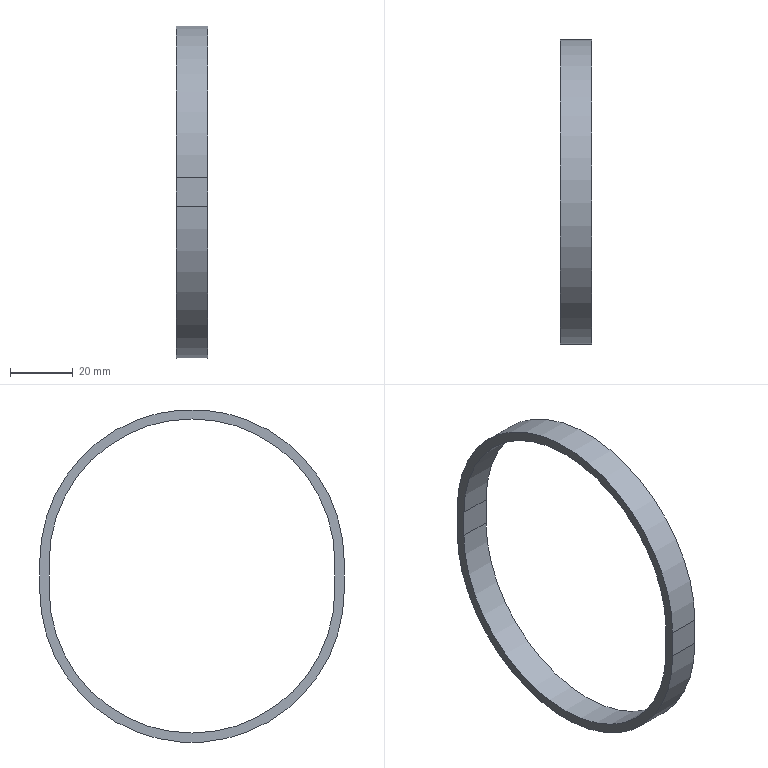Part | STEP file | 1-56.12 | 1 solid | 10 faces | box 10 x 97 x 106 mm | volume 9399 mm3 | plane 6 | cylinder 4 | commonest cylinder face diameters 91 x2 97 x2
STEP:
#1=CARTESIAN_POINT('',(0.,0.,0.));
#2=DIRECTION('',(0.,0.,1.));
#3=DIRECTION('',(1.,0.,0.));
#4=AXIS2_PLACEMENT_3D('',#1,#2,#3);
#5=CARTESIAN_POINT('',(0.,-48.5,0.));
#6=VERTEX_POINT('',#5);
#7=CARTESIAN_POINT('',(0.,-48.5,-9.));
#8=VERTEX_POINT('',#7);
#9=CARTESIAN_POINT('',(0.,-48.5,0.));
#10=DIRECTION('',(0.,0.,-1.));
#11=VECTOR('',#10,1.);
#12=LINE('',#9,#11);
#13=CARTESIAN_POINT('',(0.,4.5,-4.5));
#14=DIRECTION('',(1.,0.,0.));
#15=DIRECTION('',(0.,1.,0.));
#16=AXIS2_PLACEMENT_3D('',#13,#14,#15);
#17=PLANE('',#16);
#18=CARTESIAN_POINT('',(-53.,4.5));
#19=DIRECTION('',(0.,-1.));
#20=VECTOR('',#19,1.);
#21=LINE('',#18,#20);
#22=(GEOMETRIC_REPRESENTATION_CONTEXT(2)PARAMETRIC_REPRESENTATION_CONTEXT()REPRESENTATION_CONTEXT('',''));
#23=DEFINITIONAL_REPRESENTATION('',(#21),#22);
#24=PCURVE('',#17,#23);
#25=CARTESIAN_POINT('',(5.,-48.5,-4.5));
#26=DIRECTION('',(0.,-1.,0.));
#27=DIRECTION('',(0.,0.,-1.));
#28=AXIS2_PLACEMENT_3D('',#25,#26,#27);
#29=PLANE('',#28);
#30=CARTESIAN_POINT('',(-4.5,-5.));
#31=DIRECTION('',(1.,0.));
#32=VECTOR('',#31,1.);
#33=LINE('',#30,#32);
#34=(GEOMETRIC_REPRESENTATION_CONTEXT(2)PARAMETRIC_REPRESENTATION_CONTEXT()REPRESENTATION_CONTEXT('',''));
#35=DEFINITIONAL_REPRESENTATION('',(#33),#34);
#36=PCURVE('',#29,#35);
#37=SURFACE_CURVE('',#12,(#24,#36),.PCURVE_S1.);
#38=EDGE_CURVE('',#6,#8,#37,.T.);
#39=ORIENTED_EDGE('',*,*,#38,.T.);
#40=CARTESIAN_POINT('',(0.,48.5,-9.));
#41=VERTEX_POINT('',#40);
#42=CARTESIAN_POINT('',(0.,0.,-9.));
#43=DIRECTION('',(1.,0.,0.));
#44=DIRECTION('',(0.,-1.,0.));
#45=AXIS2_PLACEMENT_3D('',#42,#43,#44);
#46=CIRCLE('',#45,48.5);
#47=CARTESIAN_POINT('',(-4.5,-4.5));
#48=DIRECTION('',(-1.,0.));
#49=AXIS2_PLACEMENT_2D('',#47,#48);
#50=CIRCLE('',#49,48.5);
#51=(GEOMETRIC_REPRESENTATION_CONTEXT(2)PARAMETRIC_REPRESENTATION_CONTEXT()REPRESENTATION_CONTEXT('',''));
#52=DEFINITIONAL_REPRESENTATION('',(#50),#51);
#53=PCURVE('',#17,#52);
#54=CARTESIAN_POINT('',(0.,0.,-9.));
#55=DIRECTION('',(1.,0.,0.));
#56=DIRECTION('',(0.,-1.,0.));
#57=AXIS2_PLACEMENT_3D('',#54,#55,#56);
#58=CYLINDRICAL_SURFACE('',#57,48.5);
#59=CARTESIAN_POINT('',(0.,0.));
#60=DIRECTION('',(1.,0.));
#61=VECTOR('',#60,1.);
#62=LINE('',#59,#61);
#63=(GEOMETRIC_REPRESENTATION_CONTEXT(2)PARAMETRIC_REPRESENTATION_CONTEXT()REPRESENTATION_CONTEXT('',''));
#64=DEFINITIONAL_REPRESENTATION('',(#62),#63);
#65=PCURVE('',#58,#64);
#66=SURFACE_CURVE('',#46,(#53,#65),.PCURVE_S1.);
#67=EDGE_CURVE('',#8,#41,#66,.T.);
#68=ORIENTED_EDGE('',*,*,#67,.T.);
#69=CARTESIAN_POINT('',(0.,48.5,0.));
#70=VERTEX_POINT('',#69);
#71=CARTESIAN_POINT('',(0.,48.5,-9.));
#72=DIRECTION('',(0.,0.,1.));
#73=VECTOR('',#72,1.);
#74=LINE('',#71,#73);
#75=CARTESIAN_POINT('',(44.,-4.5));
#76=DIRECTION('',(0.,1.));
#77=VECTOR('',#76,1.);
#78=LINE('',#75,#77);
#79=(GEOMETRIC_REPRESENTATION_CONTEXT(2)PARAMETRIC_REPRESENTATION_CONTEXT()REPRESENTATION_CONTEXT('',''));
#80=DEFINITIONAL_REPRESENTATION('',(#78),#79);
#81=PCURVE('',#17,#80);
#82=CARTESIAN_POINT('',(5.,48.5,-4.5));
#83=DIRECTION('',(0.,1.,0.));
#84=DIRECTION('',(0.,0.,1.));
#85=AXIS2_PLACEMENT_3D('',#82,#83,#84);
#86=PLANE('',#85);
#87=CARTESIAN_POINT('',(-4.5,-5.));
#88=DIRECTION('',(1.,0.));
#89=VECTOR('',#88,1.);
#90=LINE('',#87,#89);
#91=(GEOMETRIC_REPRESENTATION_CONTEXT(2)PARAMETRIC_REPRESENTATION_CONTEXT()REPRESENTATION_CONTEXT('',''));
#92=DEFINITIONAL_REPRESENTATION('',(#90),#91);
#93=PCURVE('',#86,#92);
#94=SURFACE_CURVE('',#74,(#81,#93),.PCURVE_S1.);
#95=EDGE_CURVE('',#41,#70,#94,.T.);
#96=ORIENTED_EDGE('',*,*,#95,.T.);
#97=CARTESIAN_POINT('',(0.,0.,0.));
#98=DIRECTION('',(1.,0.,0.));
#99=DIRECTION('',(0.,1.,0.));
#100=AXIS2_PLACEMENT_3D('',#97,#98,#99);
#101=CIRCLE('',#100,48.5);
#102=CARTESIAN_POINT('',(-4.5,4.5));
#103=DIRECTION('',(1.,0.));
#104=AXIS2_PLACEMENT_2D('',#102,#103);
#105=CIRCLE('',#104,48.5);
#106=(GEOMETRIC_REPRESENTATION_CONTEXT(2)PARAMETRIC_REPRESENTATION_CONTEXT()REPRESENTATION_CONTEXT('',''));
#107=DEFINITIONAL_REPRESENTATION('',(#105),#106);
#108=PCURVE('',#17,#107);
#109=CARTESIAN_POINT('',(0.,0.,0.));
#110=DIRECTION('',(1.,0.,0.));
#111=DIRECTION('',(0.,1.,0.));
#112=AXIS2_PLACEMENT_3D('',#109,#110,#111);
#113=CYLINDRICAL_SURFACE('',#112,48.5);
#114=CARTESIAN_POINT('',(0.,0.));
#115=DIRECTION('',(1.,0.));
#116=VECTOR('',#115,1.);
#117=LINE('',#114,#116);
#118=(GEOMETRIC_REPRESENTATION_CONTEXT(2)PARAMETRIC_REPRESENTATION_CONTEXT()REPRESENTATION_CONTEXT('',''));
#119=DEFINITIONAL_REPRESENTATION('',(#117),#118);
#120=PCURVE('',#113,#119);
#121=SURFACE_CURVE('',#101,(#108,#120),.PCURVE_S1.);
#122=EDGE_CURVE('',#70,#6,#121,.T.);
#123=ORIENTED_EDGE('',*,*,#122,.T.);
#124=EDGE_LOOP('',(#39,#68,#96,#123));
#125=FACE_BOUND('',#124,.F.);
#126=CARTESIAN_POINT('',(0.,45.5,0.));
#127=VERTEX_POINT('',#126);
#128=CARTESIAN_POINT('',(0.,45.5,-9.));
#129=VERTEX_POINT('',#128);
#130=CARTESIAN_POINT('',(0.,45.5,0.));
#131=DIRECTION('',(0.,0.,-1.));
#132=VECTOR('',#131,1.);
#133=LINE('',#130,#132);
#134=CARTESIAN_POINT('',(41.,4.5));
#135=DIRECTION('',(0.,-1.));
#136=VECTOR('',#135,1.);
#137=LINE('',#134,#136);
#138=(GEOMETRIC_REPRESENTATION_CONTEXT(2)PARAMETRIC_REPRESENTATION_CONTEXT()REPRESENTATION_CONTEXT('',''));
#139=DEFINITIONAL_REPRESENTATION('',(#137),#138);
#140=PCURVE('',#17,#139);
#141=CARTESIAN_POINT('',(5.,45.5,-4.5));
#142=DIRECTION('',(0.,-1.,0.));
#143=DIRECTION('',(0.,0.,-1.));
#144=AXIS2_PLACEMENT_3D('',#141,#142,#143);
#145=PLANE('',#144);
#146=CARTESIAN_POINT('',(-4.5,-5.));
#147=DIRECTION('',(1.,0.));
#148=VECTOR('',#147,1.);
#149=LINE('',#146,#148);
#150=(GEOMETRIC_REPRESENTATION_CONTEXT(2)PARAMETRIC_REPRESENTATION_CONTEXT()REPRESENTATION_CONTEXT('',''));
#151=DEFINITIONAL_REPRESENTATION('',(#149),#150);
#152=PCURVE('',#145,#151);
#153=SURFACE_CURVE('',#133,(#140,#152),.PCURVE_S1.);
#154=EDGE_CURVE('',#127,#129,#153,.T.);
#155=ORIENTED_EDGE('',*,*,#154,.T.);
#156=CARTESIAN_POINT('',(0.,-45.5,-9.));
#157=VERTEX_POINT('',#156);
#158=CARTESIAN_POINT('',(0.,0.,-9.));
#159=DIRECTION('',(-1.,0.,0.));
#160=DIRECTION('',(0.,1.,0.));
#161=AXIS2_PLACEMENT_3D('',#158,#159,#160);
#162=CIRCLE('',#161,45.5);
#163=CARTESIAN_POINT('',(41.,-4.5));
#164=CARTESIAN_POINT('',(41.,-83.308));
#165=CARTESIAN_POINT('',(-27.25,-43.904));
#166=CARTESIAN_POINT('',(-95.5,-4.5));
#167=CARTESIAN_POINT('',(-27.25,34.904));
#168=CARTESIAN_POINT('',(41.,74.308));
#169=CARTESIAN_POINT('',(41.,-4.5));
#170=(BOUNDED_CURVE()B_SPLINE_CURVE(2,(#163,#164,#165,#166,#167,#168,#169),.UNSPECIFIED.,.T.,.F.)B_SPLINE_CURVE_WITH_KNOTS((1,2,2,2,2,1),(-2.094,0.,2.094,4.189,6.283,8.378),.UNSPECIFIED.)CURVE()GEOMETRIC_REPRESENTATION_ITEM()RATIONAL_B_SPLINE_CURVE((1.,0.5,1.,0.5,1.,0.5,1.))REPRESENTATION_ITEM(''));
#171=(GEOMETRIC_REPRESENTATION_CONTEXT(2)PARAMETRIC_REPRESENTATION_CONTEXT()REPRESENTATION_CONTEXT('',''));
#172=DEFINITIONAL_REPRESENTATION('',(#170),#171);
#173=PCURVE('',#17,#172);
#174=CARTESIAN_POINT('',(0.,0.,-9.));
#175=DIRECTION('',(1.,0.,0.));
#176=DIRECTION('',(0.,1.,0.));
#177=AXIS2_PLACEMENT_3D('',#174,#175,#176);
#178=CYLINDRICAL_SURFACE('',#177,45.5);
#179=CARTESIAN_POINT('',(6.283,0.));
#180=DIRECTION('',(-1.,0.));
#181=VECTOR('',#180,1.);
#182=LINE('',#179,#181);
#183=(GEOMETRIC_REPRESENTATION_CONTEXT(2)PARAMETRIC_REPRESENTATION_CONTEXT()REPRESENTATION_CONTEXT('',''));
#184=DEFINITIONAL_REPRESENTATION('',(#182),#183);
#185=PCURVE('',#178,#184);
#186=SURFACE_CURVE('',#162,(#173,#185),.PCURVE_S1.);
#187=EDGE_CURVE('',#129,#157,#186,.T.);
#188=ORIENTED_EDGE('',*,*,#187,.T.);
#189=CARTESIAN_POINT('',(0.,-45.5,0.));
#190=VERTEX_POINT('',#189);
#191=CARTESIAN_POINT('',(0.,-45.5,-9.));
#192=DIRECTION('',(0.,0.,1.));
#193=VECTOR('',#192,1.);
#194=LINE('',#191,#193);
#195=CARTESIAN_POINT('',(-50.,-4.5));
#196=DIRECTION('',(0.,1.));
#197=VECTOR('',#196,1.);
#198=LINE('',#195,#197);
#199=(GEOMETRIC_REPRESENTATION_CONTEXT(2)PARAMETRIC_REPRESENTATION_CONTEXT()REPRESENTATION_CONTEXT('',''));
#200=DEFINITIONAL_REPRESENTATION('',(#198),#199);
#201=PCURVE('',#17,#200);
#202=CARTESIAN_POINT('',(5.,-45.5,-4.5));
#203=DIRECTION('',(0.,1.,0.));
#204=DIRECTION('',(0.,0.,1.));
#205=AXIS2_PLACEMENT_3D('',#202,#203,#204);
#206=PLANE('',#205);
#207=CARTESIAN_POINT('',(-4.5,-5.));
#208=DIRECTION('',(1.,0.));
#209=VECTOR('',#208,1.);
#210=LINE('',#207,#209);
#211=(GEOMETRIC_REPRESENTATION_CONTEXT(2)PARAMETRIC_REPRESENTATION_CONTEXT()REPRESENTATION_CONTEXT('',''));
#212=DEFINITIONAL_REPRESENTATION('',(#210),#211);
#213=PCURVE('',#206,#212);
#214=SURFACE_CURVE('',#194,(#201,#213),.PCURVE_S1.);
#215=EDGE_CURVE('',#157,#190,#214,.T.);
#216=ORIENTED_EDGE('',*,*,#215,.T.);
#217=CARTESIAN_POINT('',(0.,0.,0.));
#218=DIRECTION('',(-1.,0.,0.));
#219=DIRECTION('',(0.,-1.,0.));
#220=AXIS2_PLACEMENT_3D('',#217,#218,#219);
#221=CIRCLE('',#220,45.5);
#222=CARTESIAN_POINT('',(-50.,4.5));
#223=CARTESIAN_POINT('',(-50.,83.308));
#224=CARTESIAN_POINT('',(18.25,43.904));
#225=CARTESIAN_POINT('',(86.5,4.5));
#226=CARTESIAN_POINT('',(18.25,-34.904));
#227=CARTESIAN_POINT('',(-50.,-74.308));
#228=CARTESIAN_POINT('',(-50.,4.5));
#229=(BOUNDED_CURVE()B_SPLINE_CURVE(2,(#222,#223,#224,#225,#226,#227,#228),.UNSPECIFIED.,.T.,.F.)B_SPLINE_CURVE_WITH_KNOTS((1,2,2,2,2,1),(-2.094,0.,2.094,4.189,6.283,8.378),.UNSPECIFIED.)CURVE()GEOMETRIC_REPRESENTATION_ITEM()RATIONAL_B_SPLINE_CURVE((1.,0.5,1.,0.5,1.,0.5,1.))REPRESENTATION_ITEM(''));
#230=(GEOMETRIC_REPRESENTATION_CONTEXT(2)PARAMETRIC_REPRESENTATION_CONTEXT()REPRESENTATION_CONTEXT('',''));
#231=DEFINITIONAL_REPRESENTATION('',(#229),#230);
#232=PCURVE('',#17,#231);
#233=CARTESIAN_POINT('',(0.,0.,0.));
#234=DIRECTION('',(1.,0.,0.));
#235=DIRECTION('',(0.,-1.,0.));
#236=AXIS2_PLACEMENT_3D('',#233,#234,#235);
#237=CYLINDRICAL_SURFACE('',#236,45.5);
#238=CARTESIAN_POINT('',(6.283,0.));
#239=DIRECTION('',(-1.,0.));
#240=VECTOR('',#239,1.);
#241=LINE('',#238,#240);
#242=(GEOMETRIC_REPRESENTATION_CONTEXT(2)PARAMETRIC_REPRESENTATION_CONTEXT()REPRESENTATION_CONTEXT('',''));
#243=DEFINITIONAL_REPRESENTATION('',(#241),#242);
#244=PCURVE('',#237,#243);
#245=SURFACE_CURVE('',#221,(#232,#244),.PCURVE_S1.);
#246=EDGE_CURVE('',#190,#127,#245,.T.);
#247=ORIENTED_EDGE('',*,*,#246,.T.);
#248=EDGE_LOOP('',(#155,#188,#216,#247));
#249=FACE_BOUND('',#248,.F.);
#250=ADVANCED_FACE('',(#125,#249),#17,.F.);
#251=CARTESIAN_POINT('',(10.,-48.5,0.));
#252=VERTEX_POINT('',#251);
#253=CARTESIAN_POINT('',(10.,-48.5,-9.));
#254=VERTEX_POINT('',#253);
#255=CARTESIAN_POINT('',(10.,-48.5,0.));
#256=DIRECTION('',(0.,0.,-1.));
#257=VECTOR('',#256,1.);
#258=LINE('',#255,#257);
#259=CARTESIAN_POINT('',(10.,4.5,-4.5));
#260=DIRECTION('',(1.,0.,0.));
#261=DIRECTION('',(0.,1.,0.));
#262=AXIS2_PLACEMENT_3D('',#259,#260,#261);
#263=PLANE('',#262);
#264=CARTESIAN_POINT('',(-53.,4.5));
#265=DIRECTION('',(0.,-1.));
#266=VECTOR('',#265,1.);
#267=LINE('',#264,#266);
#268=(GEOMETRIC_REPRESENTATION_CONTEXT(2)PARAMETRIC_REPRESENTATION_CONTEXT()REPRESENTATION_CONTEXT('',''));
#269=DEFINITIONAL_REPRESENTATION('',(#267),#268);
#270=PCURVE('',#263,#269);
#271=CARTESIAN_POINT('',(-4.5,5.));
#272=DIRECTION('',(1.,0.));
#273=VECTOR('',#272,1.);
#274=LINE('',#271,#273);
#275=(GEOMETRIC_REPRESENTATION_CONTEXT(2)PARAMETRIC_REPRESENTATION_CONTEXT()REPRESENTATION_CONTEXT('',''));
#276=DEFINITIONAL_REPRESENTATION('',(#274),#275);
#277=PCURVE('',#29,#276);
#278=SURFACE_CURVE('',#258,(#270,#277),.PCURVE_S1.);
#279=EDGE_CURVE('',#252,#254,#278,.T.);
#280=ORIENTED_EDGE('',*,*,#279,.T.);
#281=CARTESIAN_POINT('',(10.,48.5,-9.));
#282=VERTEX_POINT('',#281);
#283=CARTESIAN_POINT('',(10.,0.,-9.));
#284=DIRECTION('',(1.,0.,0.));
#285=DIRECTION('',(0.,-1.,0.));
#286=AXIS2_PLACEMENT_3D('',#283,#284,#285);
#287=CIRCLE('',#286,48.5);
#288=CARTESIAN_POINT('',(-4.5,-4.5));
#289=DIRECTION('',(-1.,0.));
#290=AXIS2_PLACEMENT_2D('',#288,#289);
#291=CIRCLE('',#290,48.5);
#292=(GEOMETRIC_REPRESENTATION_CONTEXT(2)PARAMETRIC_REPRESENTATION_CONTEXT()REPRESENTATION_CONTEXT('',''));
#293=DEFINITIONAL_REPRESENTATION('',(#291),#292);
#294=PCURVE('',#263,#293);
#295=CARTESIAN_POINT('',(0.,10.));
#296=DIRECTION('',(1.,0.));
#297=VECTOR('',#296,1.);
#298=LINE('',#295,#297);
#299=(GEOMETRIC_REPRESENTATION_CONTEXT(2)PARAMETRIC_REPRESENTATION_CONTEXT()REPRESENTATION_CONTEXT('',''));
#300=DEFINITIONAL_REPRESENTATION('',(#298),#299);
#301=PCURVE('',#58,#300);
#302=SURFACE_CURVE('',#287,(#294,#301),.PCURVE_S1.);
#303=EDGE_CURVE('',#254,#282,#302,.T.);
#304=ORIENTED_EDGE('',*,*,#303,.T.);
#305=CARTESIAN_POINT('',(10.,48.5,0.));
#306=VERTEX_POINT('',#305);
#307=CARTESIAN_POINT('',(10.,48.5,-9.));
#308=DIRECTION('',(0.,0.,1.));
#309=VECTOR('',#308,1.);
#310=LINE('',#307,#309);
#311=CARTESIAN_POINT('',(44.,-4.5));
#312=DIRECTION('',(0.,1.));
#313=VECTOR('',#312,1.);
#314=LINE('',#311,#313);
#315=(GEOMETRIC_REPRESENTATION_CONTEXT(2)PARAMETRIC_REPRESENTATION_CONTEXT()REPRESENTATION_CONTEXT('',''));
#316=DEFINITIONAL_REPRESENTATION('',(#314),#315);
#317=PCURVE('',#263,#316);
#318=CARTESIAN_POINT('',(-4.5,5.));
#319=DIRECTION('',(1.,0.));
#320=VECTOR('',#319,1.);
#321=LINE('',#318,#320);
#322=(GEOMETRIC_REPRESENTATION_CONTEXT(2)PARAMETRIC_REPRESENTATION_CONTEXT()REPRESENTATION_CONTEXT('',''));
#323=DEFINITIONAL_REPRESENTATION('',(#321),#322);
#324=PCURVE('',#86,#323);
#325=SURFACE_CURVE('',#310,(#317,#324),.PCURVE_S1.);
#326=EDGE_CURVE('',#282,#306,#325,.T.);
#327=ORIENTED_EDGE('',*,*,#326,.T.);
#328=CARTESIAN_POINT('',(10.,0.,0.));
#329=DIRECTION('',(1.,0.,0.));
#330=DIRECTION('',(0.,1.,0.));
#331=AXIS2_PLACEMENT_3D('',#328,#329,#330);
#332=CIRCLE('',#331,48.5);
#333=CARTESIAN_POINT('',(-4.5,4.5));
#334=DIRECTION('',(1.,0.));
#335=AXIS2_PLACEMENT_2D('',#333,#334);
#336=CIRCLE('',#335,48.5);
#337=(GEOMETRIC_REPRESENTATION_CONTEXT(2)PARAMETRIC_REPRESENTATION_CONTEXT()REPRESENTATION_CONTEXT('',''));
#338=DEFINITIONAL_REPRESENTATION('',(#336),#337);
#339=PCURVE('',#263,#338);
#340=CARTESIAN_POINT('',(0.,10.));
#341=DIRECTION('',(1.,0.));
#342=VECTOR('',#341,1.);
#343=LINE('',#340,#342);
#344=(GEOMETRIC_REPRESENTATION_CONTEXT(2)PARAMETRIC_REPRESENTATION_CONTEXT()REPRESENTATION_CONTEXT('',''));
#345=DEFINITIONAL_REPRESENTATION('',(#343),#344);
#346=PCURVE('',#113,#345);
#347=SURFACE_CURVE('',#332,(#339,#346),.PCURVE_S1.);
#348=EDGE_CURVE('',#306,#252,#347,.T.);
#349=ORIENTED_EDGE('',*,*,#348,.T.);
#350=EDGE_LOOP('',(#280,#304,#327,#349));
#351=FACE_BOUND('',#350,.T.);
#352=CARTESIAN_POINT('',(10.,45.5,0.));
#353=VERTEX_POINT('',#352);
#354=CARTESIAN_POINT('',(10.,45.5,-9.));
#355=VERTEX_POINT('',#354);
#356=CARTESIAN_POINT('',(10.,45.5,0.));
#357=DIRECTION('',(0.,0.,-1.));
#358=VECTOR('',#357,1.);
#359=LINE('',#356,#358);
#360=CARTESIAN_POINT('',(41.,4.5));
#361=DIRECTION('',(0.,-1.));
#362=VECTOR('',#361,1.);
#363=LINE('',#360,#362);
#364=(GEOMETRIC_REPRESENTATION_CONTEXT(2)PARAMETRIC_REPRESENTATION_CONTEXT()REPRESENTATION_CONTEXT('',''));
#365=DEFINITIONAL_REPRESENTATION('',(#363),#364);
#366=PCURVE('',#263,#365);
#367=CARTESIAN_POINT('',(-4.5,5.));
#368=DIRECTION('',(1.,0.));
#369=VECTOR('',#368,1.);
#370=LINE('',#367,#369);
#371=(GEOMETRIC_REPRESENTATION_CONTEXT(2)PARAMETRIC_REPRESENTATION_CONTEXT()REPRESENTATION_CONTEXT('',''));
#372=DEFINITIONAL_REPRESENTATION('',(#370),#371);
#373=PCURVE('',#145,#372);
#374=SURFACE_CURVE('',#359,(#366,#373),.PCURVE_S1.);
#375=EDGE_CURVE('',#353,#355,#374,.T.);
#376=ORIENTED_EDGE('',*,*,#375,.T.);
#377=CARTESIAN_POINT('',(10.,-45.5,-9.));
#378=VERTEX_POINT('',#377);
#379=CARTESIAN_POINT('',(10.,0.,-9.));
#380=DIRECTION('',(-1.,0.,0.));
#381=DIRECTION('',(0.,1.,0.));
#382=AXIS2_PLACEMENT_3D('',#379,#380,#381);
#383=CIRCLE('',#382,45.5);
#384=CARTESIAN_POINT('',(41.,-4.5));
#385=CARTESIAN_POINT('',(41.,-83.308));
#386=CARTESIAN_POINT('',(-27.25,-43.904));
#387=CARTESIAN_POINT('',(-95.5,-4.5));
#388=CARTESIAN_POINT('',(-27.25,34.904));
#389=CARTESIAN_POINT('',(41.,74.308));
#390=CARTESIAN_POINT('',(41.,-4.5));
#391=(BOUNDED_CURVE()B_SPLINE_CURVE(2,(#384,#385,#386,#387,#388,#389,#390),.UNSPECIFIED.,.T.,.F.)B_SPLINE_CURVE_WITH_KNOTS((1,2,2,2,2,1),(-2.094,0.,2.094,4.189,6.283,8.378),.UNSPECIFIED.)CURVE()GEOMETRIC_REPRESENTATION_ITEM()RATIONAL_B_SPLINE_CURVE((1.,0.5,1.,0.5,1.,0.5,1.))REPRESENTATION_ITEM(''));
#392=(GEOMETRIC_REPRESENTATION_CONTEXT(2)PARAMETRIC_REPRESENTATION_CONTEXT()REPRESENTATION_CONTEXT('',''));
#393=DEFINITIONAL_REPRESENTATION('',(#391),#392);
#394=PCURVE('',#263,#393);
#395=CARTESIAN_POINT('',(6.283,10.));
#396=DIRECTION('',(-1.,0.));
#397=VECTOR('',#396,1.);
#398=LINE('',#395,#397);
#399=(GEOMETRIC_REPRESENTATION_CONTEXT(2)PARAMETRIC_REPRESENTATION_CONTEXT()REPRESENTATION_CONTEXT('',''));
#400=DEFINITIONAL_REPRESENTATION('',(#398),#399);
#401=PCURVE('',#178,#400);
#402=SURFACE_CURVE('',#383,(#394,#401),.PCURVE_S1.);
#403=EDGE_CURVE('',#355,#378,#402,.T.);
#404=ORIENTED_EDGE('',*,*,#403,.T.);
#405=CARTESIAN_POINT('',(10.,-45.5,0.));
#406=VERTEX_POINT('',#405);
#407=CARTESIAN_POINT('',(10.,-45.5,-9.));
#408=DIRECTION('',(0.,0.,1.));
#409=VECTOR('',#408,1.);
#410=LINE('',#407,#409);
#411=CARTESIAN_POINT('',(-50.,-4.5));
#412=DIRECTION('',(0.,1.));
#413=VECTOR('',#412,1.);
#414=LINE('',#411,#413);
#415=(GEOMETRIC_REPRESENTATION_CONTEXT(2)PARAMETRIC_REPRESENTATION_CONTEXT()REPRESENTATION_CONTEXT('',''));
#416=DEFINITIONAL_REPRESENTATION('',(#414),#415);
#417=PCURVE('',#263,#416);
#418=CARTESIAN_POINT('',(-4.5,5.));
#419=DIRECTION('',(1.,0.));
#420=VECTOR('',#419,1.);
#421=LINE('',#418,#420);
#422=(GEOMETRIC_REPRESENTATION_CONTEXT(2)PARAMETRIC_REPRESENTATION_CONTEXT()REPRESENTATION_CONTEXT('',''));
#423=DEFINITIONAL_REPRESENTATION('',(#421),#422);
#424=PCURVE('',#206,#423);
#425=SURFACE_CURVE('',#410,(#417,#424),.PCURVE_S1.);
#426=EDGE_CURVE('',#378,#406,#425,.T.);
#427=ORIENTED_EDGE('',*,*,#426,.T.);
#428=CARTESIAN_POINT('',(10.,0.,0.));
#429=DIRECTION('',(-1.,0.,0.));
#430=DIRECTION('',(0.,-1.,0.));
#431=AXIS2_PLACEMENT_3D('',#428,#429,#430);
#432=CIRCLE('',#431,45.5);
#433=CARTESIAN_POINT('',(-50.,4.5));
#434=CARTESIAN_POINT('',(-50.,83.308));
#435=CARTESIAN_POINT('',(18.25,43.904));
#436=CARTESIAN_POINT('',(86.5,4.5));
#437=CARTESIAN_POINT('',(18.25,-34.904));
#438=CARTESIAN_POINT('',(-50.,-74.308));
#439=CARTESIAN_POINT('',(-50.,4.5));
#440=(BOUNDED_CURVE()B_SPLINE_CURVE(2,(#433,#434,#435,#436,#437,#438,#439),.UNSPECIFIED.,.T.,.F.)B_SPLINE_CURVE_WITH_KNOTS((1,2,2,2,2,1),(-2.094,0.,2.094,4.189,6.283,8.378),.UNSPECIFIED.)CURVE()GEOMETRIC_REPRESENTATION_ITEM()RATIONAL_B_SPLINE_CURVE((1.,0.5,1.,0.5,1.,0.5,1.))REPRESENTATION_ITEM(''));
#441=(GEOMETRIC_REPRESENTATION_CONTEXT(2)PARAMETRIC_REPRESENTATION_CONTEXT()REPRESENTATION_CONTEXT('',''));
#442=DEFINITIONAL_REPRESENTATION('',(#440),#441);
#443=PCURVE('',#263,#442);
#444=CARTESIAN_POINT('',(6.283,10.));
#445=DIRECTION('',(-1.,0.));
#446=VECTOR('',#445,1.);
#447=LINE('',#444,#446);
#448=(GEOMETRIC_REPRESENTATION_CONTEXT(2)PARAMETRIC_REPRESENTATION_CONTEXT()REPRESENTATION_CONTEXT('',''));
#449=DEFINITIONAL_REPRESENTATION('',(#447),#448);
#450=PCURVE('',#237,#449);
#451=SURFACE_CURVE('',#432,(#443,#450),.PCURVE_S1.);
#452=EDGE_CURVE('',#406,#353,#451,.T.);
#453=ORIENTED_EDGE('',*,*,#452,.T.);
#454=EDGE_LOOP('',(#376,#404,#427,#453));
#455=FACE_BOUND('',#454,.T.);
#456=ADVANCED_FACE('',(#351,#455),#263,.T.);
#457=ORIENTED_EDGE('',*,*,#38,.T.);
#458=CARTESIAN_POINT('',(0.,-48.5,-9.));
#459=DIRECTION('',(1.,0.,0.));
#460=VECTOR('',#459,1.);
#461=LINE('',#458,#460);
#462=CARTESIAN_POINT('',(4.5,-5.));
#463=DIRECTION('',(0.,1.));
#464=VECTOR('',#463,1.);
#465=LINE('',#462,#464);
#466=(GEOMETRIC_REPRESENTATION_CONTEXT(2)PARAMETRIC_REPRESENTATION_CONTEXT()REPRESENTATION_CONTEXT('',''));
#467=DEFINITIONAL_REPRESENTATION('',(#465),#466);
#468=PCURVE('',#29,#467);
#469=CARTESIAN_POINT('',(0.,0.));
#470=DIRECTION('',(0.,1.));
#471=VECTOR('',#470,1.);
#472=LINE('',#469,#471);
#473=(GEOMETRIC_REPRESENTATION_CONTEXT(2)PARAMETRIC_REPRESENTATION_CONTEXT()REPRESENTATION_CONTEXT('',''));
#474=DEFINITIONAL_REPRESENTATION('',(#472),#473);
#475=PCURVE('',#58,#474);
#476=SURFACE_CURVE('',#461,(#468,#475),.PCURVE_S1.);
#477=EDGE_CURVE('',#8,#254,#476,.T.);
#478=ORIENTED_EDGE('',*,*,#477,.T.);
#479=ORIENTED_EDGE('',*,*,#279,.F.);
#480=CARTESIAN_POINT('',(0.,-48.5,0.));
#481=DIRECTION('',(1.,0.,0.));
#482=VECTOR('',#481,1.);
#483=LINE('',#480,#482);
#484=CARTESIAN_POINT('',(-4.5,-5.));
#485=DIRECTION('',(0.,1.));
#486=VECTOR('',#485,1.);
#487=LINE('',#484,#486);
#488=(GEOMETRIC_REPRESENTATION_CONTEXT(2)PARAMETRIC_REPRESENTATION_CONTEXT()REPRESENTATION_CONTEXT('',''));
#489=DEFINITIONAL_REPRESENTATION('',(#487),#488);
#490=PCURVE('',#29,#489);
#491=CARTESIAN_POINT('',(3.142,0.));
#492=DIRECTION('',(0.,1.));
#493=VECTOR('',#492,1.);
#494=LINE('',#491,#493);
#495=(GEOMETRIC_REPRESENTATION_CONTEXT(2)PARAMETRIC_REPRESENTATION_CONTEXT()REPRESENTATION_CONTEXT('',''));
#496=DEFINITIONAL_REPRESENTATION('',(#494),#495);
#497=PCURVE('',#113,#496);
#498=SURFACE_CURVE('',#483,(#490,#497),.PCURVE_S1.);
#499=EDGE_CURVE('',#6,#252,#498,.T.);
#500=ORIENTED_EDGE('',*,*,#499,.F.);
#501=EDGE_LOOP('',(#457,#478,#479,#500));
#502=FACE_BOUND('',#501,.T.);
#503=ADVANCED_FACE('',(#502),#29,.T.);
#504=ORIENTED_EDGE('',*,*,#67,.T.);
#505=CARTESIAN_POINT('',(0.,48.5,-9.));
#506=DIRECTION('',(1.,0.,0.));
#507=VECTOR('',#506,1.);
#508=LINE('',#505,#507);
#509=CARTESIAN_POINT('',(3.142,0.));
#510=DIRECTION('',(0.,1.));
#511=VECTOR('',#510,1.);
#512=LINE('',#509,#511);
#513=(GEOMETRIC_REPRESENTATION_CONTEXT(2)PARAMETRIC_REPRESENTATION_CONTEXT()REPRESENTATION_CONTEXT('',''));
#514=DEFINITIONAL_REPRESENTATION('',(#512),#513);
#515=PCURVE('',#58,#514);
#516=CARTESIAN_POINT('',(-4.5,-5.));
#517=DIRECTION('',(0.,1.));
#518=VECTOR('',#517,1.);
#519=LINE('',#516,#518);
#520=(GEOMETRIC_REPRESENTATION_CONTEXT(2)PARAMETRIC_REPRESENTATION_CONTEXT()REPRESENTATION_CONTEXT('',''));
#521=DEFINITIONAL_REPRESENTATION('',(#519),#520);
#522=PCURVE('',#86,#521);
#523=SURFACE_CURVE('',#508,(#515,#522),.PCURVE_S1.);
#524=EDGE_CURVE('',#41,#282,#523,.T.);
#525=ORIENTED_EDGE('',*,*,#524,.T.);
#526=ORIENTED_EDGE('',*,*,#303,.F.);
#527=ORIENTED_EDGE('',*,*,#477,.F.);
#528=EDGE_LOOP('',(#504,#525,#526,#527));
#529=FACE_BOUND('',#528,.T.);
#530=ADVANCED_FACE('',(#529),#58,.T.);
#531=ORIENTED_EDGE('',*,*,#95,.T.);
#532=CARTESIAN_POINT('',(0.,48.5,0.));
#533=DIRECTION('',(1.,0.,0.));
#534=VECTOR('',#533,1.);
#535=LINE('',#532,#534);
#536=CARTESIAN_POINT('',(4.5,-5.));
#537=DIRECTION('',(0.,1.));
#538=VECTOR('',#537,1.);
#539=LINE('',#536,#538);
#540=(GEOMETRIC_REPRESENTATION_CONTEXT(2)PARAMETRIC_REPRESENTATION_CONTEXT()REPRESENTATION_CONTEXT('',''));
#541=DEFINITIONAL_REPRESENTATION('',(#539),#540);
#542=PCURVE('',#86,#541);
#543=CARTESIAN_POINT('',(0.,0.));
#544=DIRECTION('',(0.,1.));
#545=VECTOR('',#544,1.);
#546=LINE('',#543,#545);
#547=(GEOMETRIC_REPRESENTATION_CONTEXT(2)PARAMETRIC_REPRESENTATION_CONTEXT()REPRESENTATION_CONTEXT('',''));
#548=DEFINITIONAL_REPRESENTATION('',(#546),#547);
#549=PCURVE('',#113,#548);
#550=SURFACE_CURVE('',#535,(#542,#549),.PCURVE_S1.);
#551=EDGE_CURVE('',#70,#306,#550,.T.);
#552=ORIENTED_EDGE('',*,*,#551,.T.);
#553=ORIENTED_EDGE('',*,*,#326,.F.);
#554=ORIENTED_EDGE('',*,*,#524,.F.);
#555=EDGE_LOOP('',(#531,#552,#553,#554));
#556=FACE_BOUND('',#555,.T.);
#557=ADVANCED_FACE('',(#556),#86,.T.);
#558=ORIENTED_EDGE('',*,*,#122,.T.);
#559=ORIENTED_EDGE('',*,*,#499,.T.);
#560=ORIENTED_EDGE('',*,*,#348,.F.);
#561=ORIENTED_EDGE('',*,*,#551,.F.);
#562=EDGE_LOOP('',(#558,#559,#560,#561));
#563=FACE_BOUND('',#562,.T.);
#564=ADVANCED_FACE('',(#563),#113,.T.);
#565=ORIENTED_EDGE('',*,*,#154,.T.);
#566=CARTESIAN_POINT('',(0.,45.5,-9.));
#567=DIRECTION('',(1.,0.,0.));
#568=VECTOR('',#567,1.);
#569=LINE('',#566,#568);
#570=CARTESIAN_POINT('',(4.5,-5.));
#571=DIRECTION('',(0.,1.));
#572=VECTOR('',#571,1.);
#573=LINE('',#570,#572);
#574=(GEOMETRIC_REPRESENTATION_CONTEXT(2)PARAMETRIC_REPRESENTATION_CONTEXT()REPRESENTATION_CONTEXT('',''));
#575=DEFINITIONAL_REPRESENTATION('',(#573),#574);
#576=PCURVE('',#145,#575);
#577=CARTESIAN_POINT('',(6.283,0.));
#578=DIRECTION('',(0.,1.));
#579=VECTOR('',#578,1.);
#580=LINE('',#577,#579);
#581=(GEOMETRIC_REPRESENTATION_CONTEXT(2)PARAMETRIC_REPRESENTATION_CONTEXT()REPRESENTATION_CONTEXT('',''));
#582=DEFINITIONAL_REPRESENTATION('',(#580),#581);
#583=PCURVE('',#178,#582);
#584=SURFACE_CURVE('',#569,(#576,#583),.PCURVE_S1.);
#585=EDGE_CURVE('',#129,#355,#584,.T.);
#586=ORIENTED_EDGE('',*,*,#585,.T.);
#587=ORIENTED_EDGE('',*,*,#375,.F.);
#588=CARTESIAN_POINT('',(0.,45.5,0.));
#589=DIRECTION('',(1.,0.,0.));
#590=VECTOR('',#589,1.);
#591=LINE('',#588,#590);
#592=CARTESIAN_POINT('',(-4.5,-5.));
#593=DIRECTION('',(0.,1.));
#594=VECTOR('',#593,1.);
#595=LINE('',#592,#594);
#596=(GEOMETRIC_REPRESENTATION_CONTEXT(2)PARAMETRIC_REPRESENTATION_CONTEXT()REPRESENTATION_CONTEXT('',''));
#597=DEFINITIONAL_REPRESENTATION('',(#595),#596);
#598=PCURVE('',#145,#597);
#599=CARTESIAN_POINT('',(3.142,0.));
#600=DIRECTION('',(0.,1.));
#601=VECTOR('',#600,1.);
#602=LINE('',#599,#601);
#603=(GEOMETRIC_REPRESENTATION_CONTEXT(2)PARAMETRIC_REPRESENTATION_CONTEXT()REPRESENTATION_CONTEXT('',''));
#604=DEFINITIONAL_REPRESENTATION('',(#602),#603);
#605=PCURVE('',#237,#604);
#606=SURFACE_CURVE('',#591,(#598,#605),.PCURVE_S1.);
#607=EDGE_CURVE('',#127,#353,#606,.T.);
#608=ORIENTED_EDGE('',*,*,#607,.F.);
#609=EDGE_LOOP('',(#565,#586,#587,#608));
#610=FACE_BOUND('',#609,.T.);
#611=ADVANCED_FACE('',(#610),#145,.T.);
#612=ORIENTED_EDGE('',*,*,#585,.T.);
#613=ORIENTED_EDGE('',*,*,#403,.T.);
#614=CARTESIAN_POINT('',(0.,-45.5,-9.));
#615=DIRECTION('',(1.,0.,0.));
#616=VECTOR('',#615,1.);
#617=LINE('',#614,#616);
#618=CARTESIAN_POINT('',(3.142,0.));
#619=DIRECTION('',(0.,1.));
#620=VECTOR('',#619,1.);
#621=LINE('',#618,#620);
#622=(GEOMETRIC_REPRESENTATION_CONTEXT(2)PARAMETRIC_REPRESENTATION_CONTEXT()REPRESENTATION_CONTEXT('',''));
#623=DEFINITIONAL_REPRESENTATION('',(#621),#622);
#624=PCURVE('',#178,#623);
#625=CARTESIAN_POINT('',(-4.5,-5.));
#626=DIRECTION('',(0.,1.));
#627=VECTOR('',#626,1.);
#628=LINE('',#625,#627);
#629=(GEOMETRIC_REPRESENTATION_CONTEXT(2)PARAMETRIC_REPRESENTATION_CONTEXT()REPRESENTATION_CONTEXT('',''));
#630=DEFINITIONAL_REPRESENTATION('',(#628),#629);
#631=PCURVE('',#206,#630);
#632=SURFACE_CURVE('',#617,(#624,#631),.PCURVE_S1.);
#633=EDGE_CURVE('',#157,#378,#632,.T.);
#634=ORIENTED_EDGE('',*,*,#633,.F.);
#635=ORIENTED_EDGE('',*,*,#187,.F.);
#636=EDGE_LOOP('',(#612,#613,#634,#635));
#637=FACE_BOUND('',#636,.F.);
#638=ADVANCED_FACE('',(#637),#178,.F.);
#639=ORIENTED_EDGE('',*,*,#215,.T.);
#640=CARTESIAN_POINT('',(0.,-45.5,0.));
#641=DIRECTION('',(1.,0.,0.));
#642=VECTOR('',#641,1.);
#643=LINE('',#640,#642);
#644=CARTESIAN_POINT('',(4.5,-5.));
#645=DIRECTION('',(0.,1.));
#646=VECTOR('',#645,1.);
#647=LINE('',#644,#646);
#648=(GEOMETRIC_REPRESENTATION_CONTEXT(2)PARAMETRIC_REPRESENTATION_CONTEXT()REPRESENTATION_CONTEXT('',''));
#649=DEFINITIONAL_REPRESENTATION('',(#647),#648);
#650=PCURVE('',#206,#649);
#651=CARTESIAN_POINT('',(6.283,0.));
#652=DIRECTION('',(0.,1.));
#653=VECTOR('',#652,1.);
#654=LINE('',#651,#653);
#655=(GEOMETRIC_REPRESENTATION_CONTEXT(2)PARAMETRIC_REPRESENTATION_CONTEXT()REPRESENTATION_CONTEXT('',''));
#656=DEFINITIONAL_REPRESENTATION('',(#654),#655);
#657=PCURVE('',#237,#656);
#658=SURFACE_CURVE('',#643,(#650,#657),.PCURVE_S1.);
#659=EDGE_CURVE('',#190,#406,#658,.T.);
#660=ORIENTED_EDGE('',*,*,#659,.T.);
#661=ORIENTED_EDGE('',*,*,#426,.F.);
#662=ORIENTED_EDGE('',*,*,#633,.F.);
#663=EDGE_LOOP('',(#639,#660,#661,#662));
#664=FACE_BOUND('',#663,.T.);
#665=ADVANCED_FACE('',(#664),#206,.T.);
#666=ORIENTED_EDGE('',*,*,#659,.T.);
#667=ORIENTED_EDGE('',*,*,#452,.T.);
#668=ORIENTED_EDGE('',*,*,#607,.F.);
#669=ORIENTED_EDGE('',*,*,#246,.F.);
#670=EDGE_LOOP('',(#666,#667,#668,#669));
#671=FACE_BOUND('',#670,.F.);
#672=ADVANCED_FACE('',(#671),#237,.F.);
#673=CLOSED_SHELL('',(#250,#456,#503,#530,#557,#564,#611,#638,#665,#672));
#674=MANIFOLD_SOLID_BREP('',#673);
#675=(LENGTH_UNIT()NAMED_UNIT(*)SI_UNIT(.MILLI.,.METRE.));
#676=UNCERTAINTY_MEASURE_WITH_UNIT(LENGTH_MEASURE(0.0000001),#675,'','');
#677=(NAMED_UNIT(*)PLANE_ANGLE_UNIT()SI_UNIT($,.RADIAN.));
#678=(NAMED_UNIT(*)SI_UNIT($,.STERADIAN.)SOLID_ANGLE_UNIT());
#679=(GEOMETRIC_REPRESENTATION_CONTEXT(3)GLOBAL_UNCERTAINTY_ASSIGNED_CONTEXT((#676))GLOBAL_UNIT_ASSIGNED_CONTEXT((#675,#677,#678))REPRESENTATION_CONTEXT('',''));
#680=ADVANCED_BREP_SHAPE_REPRESENTATION('',(#4,#674),#679);